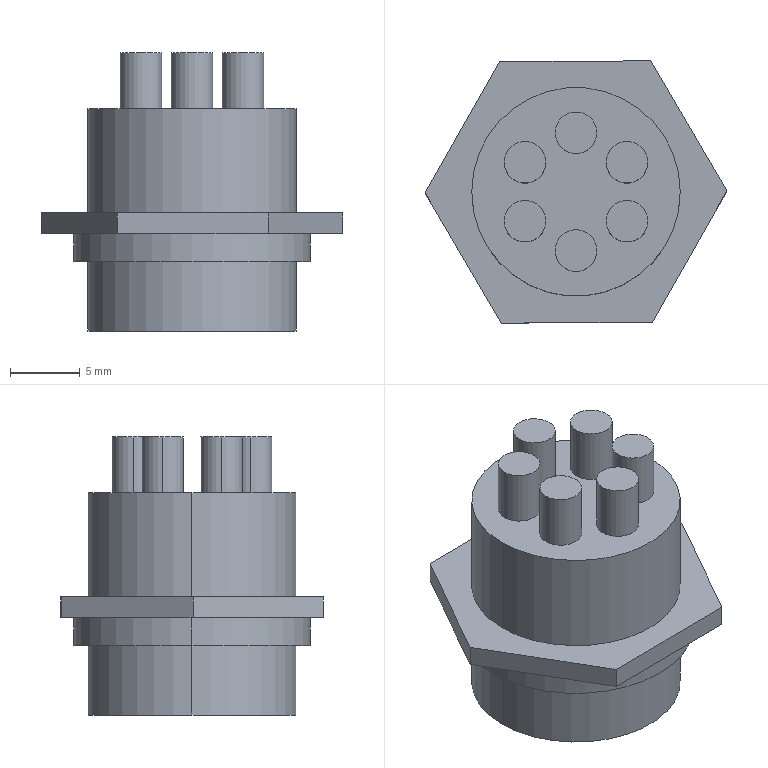Part | STEP file | 航插-1 | 1 solid | 56 faces | box 21.708 x 18.872 x 20 mm | volume 2692 mm3 | cylinder 32 | plane 24 | commonest cylinder face diameters 3 x24 15 x4 14 x2 17 x2
STEP:
#1=CARTESIAN_POINT('',(-7.5,0.,16.));
#2=VERTEX_POINT('',#1);
#3=CARTESIAN_POINT('',(7.5,0.,16.));
#4=VERTEX_POINT('',#3);
#5=CARTESIAN_POINT('',(0.,0.,16.));
#6=DIRECTION('',(0.,0.,-1.));
#7=DIRECTION('',(-1.,0.,0.));
#8=AXIS2_PLACEMENT_3D('',#5,#6,#7);
#9=CIRCLE('',#8,7.5);
#10=EDGE_CURVE('',#2,#4,#9,.T.);
#11=ORIENTED_EDGE('',*,*,#10,.T.);
#12=CARTESIAN_POINT('',(7.5,0.,8.5));
#13=VERTEX_POINT('',#12);
#14=CARTESIAN_POINT('',(7.5,0.,16.));
#15=DIRECTION('',(0.,0.,-1.));
#16=VECTOR('',#15,1000.);
#17=LINE('',#14,#16);
#18=EDGE_CURVE('',#4,#13,#17,.T.);
#19=ORIENTED_EDGE('',*,*,#18,.T.);
#20=CARTESIAN_POINT('',(-7.5,0.,8.5));
#21=VERTEX_POINT('',#20);
#22=CARTESIAN_POINT('',(0.,0.,8.5));
#23=DIRECTION('',(0.,0.,1.));
#24=DIRECTION('',(-1.,0.,0.));
#25=AXIS2_PLACEMENT_3D('',#22,#23,#24);
#26=CIRCLE('',#25,7.5);
#27=EDGE_CURVE('',#13,#21,#26,.T.);
#28=ORIENTED_EDGE('',*,*,#27,.T.);
#29=CARTESIAN_POINT('',(-7.5,0.,16.));
#30=DIRECTION('',(0.,0.,-1.));
#31=VECTOR('',#30,1000.);
#32=LINE('',#29,#31);
#33=EDGE_CURVE('',#2,#21,#32,.T.);
#34=ORIENTED_EDGE('',*,*,#33,.F.);
#35=EDGE_LOOP('',(#11,#19,#28,#34));
#36=FACE_OUTER_BOUND('',#35,.T.);
#37=CARTESIAN_POINT('',(0.,0.,16.));
#38=DIRECTION('',(0.,0.,-1.));
#39=DIRECTION('',(-1.,0.,0.));
#40=AXIS2_PLACEMENT_3D('',#37,#38,#39);
#41=CYLINDRICAL_SURFACE('',#40,7.5);
#42=ADVANCED_FACE('',(#36),#41,.T.);
#43=CARTESIAN_POINT('',(-5.17,2.119,20.));
#44=VERTEX_POINT('',#43);
#45=CARTESIAN_POINT('',(-2.17,2.119,20.));
#46=VERTEX_POINT('',#45);
#47=CARTESIAN_POINT('',(-3.67,2.119,20.));
#48=DIRECTION('',(0.,0.,-1.));
#49=DIRECTION('',(-1.,0.,0.));
#50=AXIS2_PLACEMENT_3D('',#47,#48,#49);
#51=CIRCLE('',#50,1.5);
#52=EDGE_CURVE('',#44,#46,#51,.T.);
#53=ORIENTED_EDGE('',*,*,#52,.T.);
#54=CARTESIAN_POINT('',(-2.17,2.119,16.));
#55=VERTEX_POINT('',#54);
#56=CARTESIAN_POINT('',(-2.17,2.119,20.));
#57=DIRECTION('',(0.,0.,-1.));
#58=VECTOR('',#57,1000.);
#59=LINE('',#56,#58);
#60=EDGE_CURVE('',#46,#55,#59,.T.);
#61=ORIENTED_EDGE('',*,*,#60,.T.);
#62=CARTESIAN_POINT('',(-5.17,2.119,16.));
#63=VERTEX_POINT('',#62);
#64=CARTESIAN_POINT('',(-3.67,2.119,16.));
#65=DIRECTION('',(0.,0.,-1.));
#66=DIRECTION('',(-1.,0.,0.));
#67=AXIS2_PLACEMENT_3D('',#64,#65,#66);
#68=CIRCLE('',#67,1.5);
#69=EDGE_CURVE('',#63,#55,#68,.T.);
#70=ORIENTED_EDGE('',*,*,#69,.F.);
#71=CARTESIAN_POINT('',(-5.17,2.119,20.));
#72=DIRECTION('',(0.,0.,-1.));
#73=VECTOR('',#72,1000.);
#74=LINE('',#71,#73);
#75=EDGE_CURVE('',#44,#63,#74,.T.);
#76=ORIENTED_EDGE('',*,*,#75,.F.);
#77=EDGE_LOOP('',(#53,#61,#70,#76));
#78=FACE_OUTER_BOUND('',#77,.T.);
#79=CARTESIAN_POINT('',(-3.67,2.119,20.));
#80=DIRECTION('',(0.,0.,-1.));
#81=DIRECTION('',(-1.,0.,0.));
#82=AXIS2_PLACEMENT_3D('',#79,#80,#81);
#83=CYLINDRICAL_SURFACE('',#82,1.5);
#84=ADVANCED_FACE('',(#78),#83,.T.);
#85=CARTESIAN_POINT('',(-5.17,-2.119,20.));
#86=VERTEX_POINT('',#85);
#87=CARTESIAN_POINT('',(-2.17,-2.119,20.));
#88=VERTEX_POINT('',#87);
#89=CARTESIAN_POINT('',(-3.67,-2.119,20.));
#90=DIRECTION('',(0.,0.,-1.));
#91=DIRECTION('',(-1.,0.,0.));
#92=AXIS2_PLACEMENT_3D('',#89,#90,#91);
#93=CIRCLE('',#92,1.5);
#94=EDGE_CURVE('',#86,#88,#93,.T.);
#95=ORIENTED_EDGE('',*,*,#94,.T.);
#96=CARTESIAN_POINT('',(-2.17,-2.119,16.));
#97=VERTEX_POINT('',#96);
#98=CARTESIAN_POINT('',(-2.17,-2.119,20.));
#99=DIRECTION('',(0.,0.,-1.));
#100=VECTOR('',#99,1000.);
#101=LINE('',#98,#100);
#102=EDGE_CURVE('',#88,#97,#101,.T.);
#103=ORIENTED_EDGE('',*,*,#102,.T.);
#104=CARTESIAN_POINT('',(-5.17,-2.119,16.));
#105=VERTEX_POINT('',#104);
#106=CARTESIAN_POINT('',(-3.67,-2.119,16.));
#107=DIRECTION('',(0.,0.,-1.));
#108=DIRECTION('',(-1.,0.,0.));
#109=AXIS2_PLACEMENT_3D('',#106,#107,#108);
#110=CIRCLE('',#109,1.5);
#111=EDGE_CURVE('',#105,#97,#110,.T.);
#112=ORIENTED_EDGE('',*,*,#111,.F.);
#113=CARTESIAN_POINT('',(-5.17,-2.119,20.));
#114=DIRECTION('',(0.,0.,-1.));
#115=VECTOR('',#114,1000.);
#116=LINE('',#113,#115);
#117=EDGE_CURVE('',#86,#105,#116,.T.);
#118=ORIENTED_EDGE('',*,*,#117,.F.);
#119=EDGE_LOOP('',(#95,#103,#112,#118));
#120=FACE_OUTER_BOUND('',#119,.T.);
#121=CARTESIAN_POINT('',(-3.67,-2.119,20.));
#122=DIRECTION('',(0.,0.,-1.));
#123=DIRECTION('',(-1.,0.,0.));
#124=AXIS2_PLACEMENT_3D('',#121,#122,#123);
#125=CYLINDRICAL_SURFACE('',#124,1.5);
#126=ADVANCED_FACE('',(#120),#125,.T.);
#127=CARTESIAN_POINT('',(-1.5,-4.238,20.));
#128=VERTEX_POINT('',#127);
#129=CARTESIAN_POINT('',(1.5,-4.238,20.));
#130=VERTEX_POINT('',#129);
#131=CARTESIAN_POINT('',(0.,-4.238,20.));
#132=DIRECTION('',(0.,0.,-1.));
#133=DIRECTION('',(-1.,0.,0.));
#134=AXIS2_PLACEMENT_3D('',#131,#132,#133);
#135=CIRCLE('',#134,1.5);
#136=EDGE_CURVE('',#128,#130,#135,.T.);
#137=ORIENTED_EDGE('',*,*,#136,.T.);
#138=CARTESIAN_POINT('',(1.5,-4.238,16.));
#139=VERTEX_POINT('',#138);
#140=CARTESIAN_POINT('',(1.5,-4.238,20.));
#141=DIRECTION('',(0.,0.,-1.));
#142=VECTOR('',#141,1000.);
#143=LINE('',#140,#142);
#144=EDGE_CURVE('',#130,#139,#143,.T.);
#145=ORIENTED_EDGE('',*,*,#144,.T.);
#146=CARTESIAN_POINT('',(-1.5,-4.238,16.));
#147=VERTEX_POINT('',#146);
#148=CARTESIAN_POINT('',(0.,-4.238,16.));
#149=DIRECTION('',(0.,0.,-1.));
#150=DIRECTION('',(-1.,0.,0.));
#151=AXIS2_PLACEMENT_3D('',#148,#149,#150);
#152=CIRCLE('',#151,1.5);
#153=EDGE_CURVE('',#147,#139,#152,.T.);
#154=ORIENTED_EDGE('',*,*,#153,.F.);
#155=CARTESIAN_POINT('',(-1.5,-4.238,20.));
#156=DIRECTION('',(0.,0.,-1.));
#157=VECTOR('',#156,1000.);
#158=LINE('',#155,#157);
#159=EDGE_CURVE('',#128,#147,#158,.T.);
#160=ORIENTED_EDGE('',*,*,#159,.F.);
#161=EDGE_LOOP('',(#137,#145,#154,#160));
#162=FACE_OUTER_BOUND('',#161,.T.);
#163=CARTESIAN_POINT('',(0.,-4.238,20.));
#164=DIRECTION('',(0.,0.,-1.));
#165=DIRECTION('',(-1.,0.,0.));
#166=AXIS2_PLACEMENT_3D('',#163,#164,#165);
#167=CYLINDRICAL_SURFACE('',#166,1.5);
#168=ADVANCED_FACE('',(#162),#167,.T.);
#169=CARTESIAN_POINT('',(2.17,-2.119,20.));
#170=VERTEX_POINT('',#169);
#171=CARTESIAN_POINT('',(5.17,-2.119,20.));
#172=VERTEX_POINT('',#171);
#173=CARTESIAN_POINT('',(3.67,-2.119,20.));
#174=DIRECTION('',(0.,0.,-1.));
#175=DIRECTION('',(-1.,0.,0.));
#176=AXIS2_PLACEMENT_3D('',#173,#174,#175);
#177=CIRCLE('',#176,1.5);
#178=EDGE_CURVE('',#170,#172,#177,.T.);
#179=ORIENTED_EDGE('',*,*,#178,.T.);
#180=CARTESIAN_POINT('',(5.17,-2.119,16.));
#181=VERTEX_POINT('',#180);
#182=CARTESIAN_POINT('',(5.17,-2.119,20.));
#183=DIRECTION('',(0.,0.,-1.));
#184=VECTOR('',#183,1000.);
#185=LINE('',#182,#184);
#186=EDGE_CURVE('',#172,#181,#185,.T.);
#187=ORIENTED_EDGE('',*,*,#186,.T.);
#188=CARTESIAN_POINT('',(2.17,-2.119,16.));
#189=VERTEX_POINT('',#188);
#190=CARTESIAN_POINT('',(3.67,-2.119,16.));
#191=DIRECTION('',(0.,0.,-1.));
#192=DIRECTION('',(-1.,0.,0.));
#193=AXIS2_PLACEMENT_3D('',#190,#191,#192);
#194=CIRCLE('',#193,1.5);
#195=EDGE_CURVE('',#189,#181,#194,.T.);
#196=ORIENTED_EDGE('',*,*,#195,.F.);
#197=CARTESIAN_POINT('',(2.17,-2.119,20.));
#198=DIRECTION('',(0.,0.,-1.));
#199=VECTOR('',#198,1000.);
#200=LINE('',#197,#199);
#201=EDGE_CURVE('',#170,#189,#200,.T.);
#202=ORIENTED_EDGE('',*,*,#201,.F.);
#203=EDGE_LOOP('',(#179,#187,#196,#202));
#204=FACE_OUTER_BOUND('',#203,.T.);
#205=CARTESIAN_POINT('',(3.67,-2.119,20.));
#206=DIRECTION('',(0.,0.,-1.));
#207=DIRECTION('',(-1.,0.,0.));
#208=AXIS2_PLACEMENT_3D('',#205,#206,#207);
#209=CYLINDRICAL_SURFACE('',#208,1.5);
#210=ADVANCED_FACE('',(#204),#209,.T.);
#211=CARTESIAN_POINT('',(2.17,2.119,20.));
#212=VERTEX_POINT('',#211);
#213=CARTESIAN_POINT('',(5.17,2.119,20.));
#214=VERTEX_POINT('',#213);
#215=CARTESIAN_POINT('',(3.67,2.119,20.));
#216=DIRECTION('',(0.,0.,-1.));
#217=DIRECTION('',(-1.,0.,0.));
#218=AXIS2_PLACEMENT_3D('',#215,#216,#217);
#219=CIRCLE('',#218,1.5);
#220=EDGE_CURVE('',#212,#214,#219,.T.);
#221=ORIENTED_EDGE('',*,*,#220,.T.);
#222=CARTESIAN_POINT('',(5.17,2.119,16.));
#223=VERTEX_POINT('',#222);
#224=CARTESIAN_POINT('',(5.17,2.119,20.));
#225=DIRECTION('',(0.,0.,-1.));
#226=VECTOR('',#225,1000.);
#227=LINE('',#224,#226);
#228=EDGE_CURVE('',#214,#223,#227,.T.);
#229=ORIENTED_EDGE('',*,*,#228,.T.);
#230=CARTESIAN_POINT('',(2.17,2.119,16.));
#231=VERTEX_POINT('',#230);
#232=CARTESIAN_POINT('',(3.67,2.119,16.));
#233=DIRECTION('',(0.,0.,-1.));
#234=DIRECTION('',(-1.,0.,0.));
#235=AXIS2_PLACEMENT_3D('',#232,#233,#234);
#236=CIRCLE('',#235,1.5);
#237=EDGE_CURVE('',#231,#223,#236,.T.);
#238=ORIENTED_EDGE('',*,*,#237,.F.);
#239=CARTESIAN_POINT('',(2.17,2.119,20.));
#240=DIRECTION('',(0.,0.,-1.));
#241=VECTOR('',#240,1000.);
#242=LINE('',#239,#241);
#243=EDGE_CURVE('',#212,#231,#242,.T.);
#244=ORIENTED_EDGE('',*,*,#243,.F.);
#245=EDGE_LOOP('',(#221,#229,#238,#244));
#246=FACE_OUTER_BOUND('',#245,.T.);
#247=CARTESIAN_POINT('',(3.67,2.119,20.));
#248=DIRECTION('',(0.,0.,-1.));
#249=DIRECTION('',(-1.,0.,0.));
#250=AXIS2_PLACEMENT_3D('',#247,#248,#249);
#251=CYLINDRICAL_SURFACE('',#250,1.5);
#252=ADVANCED_FACE('',(#246),#251,.T.);
#253=CARTESIAN_POINT('',(-1.5,4.238,20.));
#254=VERTEX_POINT('',#253);
#255=CARTESIAN_POINT('',(1.5,4.238,20.));
#256=VERTEX_POINT('',#255);
#257=CARTESIAN_POINT('',(0.,4.238,20.));
#258=DIRECTION('',(0.,0.,-1.));
#259=DIRECTION('',(-1.,0.,0.));
#260=AXIS2_PLACEMENT_3D('',#257,#258,#259);
#261=CIRCLE('',#260,1.5);
#262=EDGE_CURVE('',#254,#256,#261,.T.);
#263=ORIENTED_EDGE('',*,*,#262,.T.);
#264=CARTESIAN_POINT('',(1.5,4.238,16.));
#265=VERTEX_POINT('',#264);
#266=CARTESIAN_POINT('',(1.5,4.238,20.));
#267=DIRECTION('',(0.,0.,-1.));
#268=VECTOR('',#267,1000.);
#269=LINE('',#266,#268);
#270=EDGE_CURVE('',#256,#265,#269,.T.);
#271=ORIENTED_EDGE('',*,*,#270,.T.);
#272=CARTESIAN_POINT('',(-1.5,4.238,16.));
#273=VERTEX_POINT('',#272);
#274=CARTESIAN_POINT('',(0.,4.238,16.));
#275=DIRECTION('',(0.,0.,-1.));
#276=DIRECTION('',(-1.,0.,0.));
#277=AXIS2_PLACEMENT_3D('',#274,#275,#276);
#278=CIRCLE('',#277,1.5);
#279=EDGE_CURVE('',#273,#265,#278,.T.);
#280=ORIENTED_EDGE('',*,*,#279,.F.);
#281=CARTESIAN_POINT('',(-1.5,4.238,20.));
#282=DIRECTION('',(0.,0.,-1.));
#283=VECTOR('',#282,1000.);
#284=LINE('',#281,#283);
#285=EDGE_CURVE('',#254,#273,#284,.T.);
#286=ORIENTED_EDGE('',*,*,#285,.F.);
#287=EDGE_LOOP('',(#263,#271,#280,#286));
#288=FACE_OUTER_BOUND('',#287,.T.);
#289=CARTESIAN_POINT('',(0.,4.238,20.));
#290=DIRECTION('',(0.,0.,-1.));
#291=DIRECTION('',(-1.,0.,0.));
#292=AXIS2_PLACEMENT_3D('',#289,#290,#291);
#293=CYLINDRICAL_SURFACE('',#292,1.5);
#294=ADVANCED_FACE('',(#288),#293,.T.);
#295=CARTESIAN_POINT('',(-8.5,0.,7.));
#296=VERTEX_POINT('',#295);
#297=CARTESIAN_POINT('',(8.5,0.,7.));
#298=VERTEX_POINT('',#297);
#299=CARTESIAN_POINT('',(0.,0.,7.));
#300=DIRECTION('',(0.,0.,-1.));
#301=DIRECTION('',(-1.,0.,0.));
#302=AXIS2_PLACEMENT_3D('',#299,#300,#301);
#303=CIRCLE('',#302,8.5);
#304=EDGE_CURVE('',#296,#298,#303,.T.);
#305=ORIENTED_EDGE('',*,*,#304,.T.);
#306=CARTESIAN_POINT('',(8.5,0.,5.));
#307=VERTEX_POINT('',#306);
#308=CARTESIAN_POINT('',(8.5,0.,7.));
#309=DIRECTION('',(0.,0.,-1.));
#310=VECTOR('',#309,1000.);
#311=LINE('',#308,#310);
#312=EDGE_CURVE('',#298,#307,#311,.T.);
#313=ORIENTED_EDGE('',*,*,#312,.T.);
#314=CARTESIAN_POINT('',(-8.5,0.,5.));
#315=VERTEX_POINT('',#314);
#316=CARTESIAN_POINT('',(0.,0.,5.));
#317=DIRECTION('',(0.,0.,1.));
#318=DIRECTION('',(-1.,0.,0.));
#319=AXIS2_PLACEMENT_3D('',#316,#317,#318);
#320=CIRCLE('',#319,8.5);
#321=EDGE_CURVE('',#307,#315,#320,.T.);
#322=ORIENTED_EDGE('',*,*,#321,.T.);
#323=CARTESIAN_POINT('',(-8.5,0.,7.));
#324=DIRECTION('',(0.,0.,-1.));
#325=VECTOR('',#324,1000.);
#326=LINE('',#323,#325);
#327=EDGE_CURVE('',#296,#315,#326,.T.);
#328=ORIENTED_EDGE('',*,*,#327,.F.);
#329=EDGE_LOOP('',(#305,#313,#322,#328));
#330=FACE_OUTER_BOUND('',#329,.T.);
#331=CARTESIAN_POINT('',(0.,0.,7.));
#332=DIRECTION('',(0.,0.,-1.));
#333=DIRECTION('',(-1.,0.,0.));
#334=AXIS2_PLACEMENT_3D('',#331,#332,#333);
#335=CYLINDRICAL_SURFACE('',#334,8.5);
#336=ADVANCED_FACE('',(#330),#335,.T.);
#337=CARTESIAN_POINT('',(-7.5,0.,5.));
#338=VERTEX_POINT('',#337);
#339=CARTESIAN_POINT('',(7.5,0.,5.));
#340=VERTEX_POINT('',#339);
#341=CARTESIAN_POINT('',(0.,0.,5.));
#342=DIRECTION('',(0.,0.,-1.));
#343=DIRECTION('',(-1.,0.,0.));
#344=AXIS2_PLACEMENT_3D('',#341,#342,#343);
#345=CIRCLE('',#344,7.5);
#346=EDGE_CURVE('',#338,#340,#345,.T.);
#347=ORIENTED_EDGE('',*,*,#346,.T.);
#348=CARTESIAN_POINT('',(7.5,0.,0.));
#349=VERTEX_POINT('',#348);
#350=CARTESIAN_POINT('',(7.5,0.,5.));
#351=DIRECTION('',(0.,0.,-1.));
#352=VECTOR('',#351,1000.);
#353=LINE('',#350,#352);
#354=EDGE_CURVE('',#340,#349,#353,.T.);
#355=ORIENTED_EDGE('',*,*,#354,.T.);
#356=CARTESIAN_POINT('',(-7.5,0.,0.));
#357=VERTEX_POINT('',#356);
#358=CARTESIAN_POINT('',(0.,0.,0.));
#359=DIRECTION('',(0.,0.,1.));
#360=DIRECTION('',(-1.,0.,0.));
#361=AXIS2_PLACEMENT_3D('',#358,#359,#360);
#362=CIRCLE('',#361,7.5);
#363=EDGE_CURVE('',#349,#357,#362,.T.);
#364=ORIENTED_EDGE('',*,*,#363,.T.);
#365=CARTESIAN_POINT('',(-7.5,0.,5.));
#366=DIRECTION('',(0.,0.,-1.));
#367=VECTOR('',#366,1000.);
#368=LINE('',#365,#367);
#369=EDGE_CURVE('',#338,#357,#368,.T.);
#370=ORIENTED_EDGE('',*,*,#369,.F.);
#371=EDGE_LOOP('',(#347,#355,#364,#370));
#372=FACE_OUTER_BOUND('',#371,.T.);
#373=CARTESIAN_POINT('',(0.,0.,5.));
#374=DIRECTION('',(0.,0.,-1.));
#375=DIRECTION('',(-1.,0.,0.));
#376=AXIS2_PLACEMENT_3D('',#373,#374,#375);
#377=CYLINDRICAL_SURFACE('',#376,7.5);
#378=ADVANCED_FACE('',(#372),#377,.T.);
#379=CARTESIAN_POINT('',(7.,0.,5.));
#380=VERTEX_POINT('',#379);
#381=CARTESIAN_POINT('',(-7.,0.,5.));
#382=VERTEX_POINT('',#381);
#383=CARTESIAN_POINT('',(0.,0.,5.));
#384=DIRECTION('',(0.,0.,-1.));
#385=DIRECTION('',(-1.,0.,0.));
#386=AXIS2_PLACEMENT_3D('',#383,#384,#385);
#387=CIRCLE('',#386,7.);
#388=EDGE_CURVE('',#380,#382,#387,.T.);
#389=ORIENTED_EDGE('',*,*,#388,.F.);
#390=CARTESIAN_POINT('',(7.,0.,0.));
#391=VERTEX_POINT('',#390);
#392=CARTESIAN_POINT('',(7.,0.,5.));
#393=DIRECTION('',(0.,0.,-1.));
#394=VECTOR('',#393,1000.);
#395=LINE('',#392,#394);
#396=EDGE_CURVE('',#380,#391,#395,.T.);
#397=ORIENTED_EDGE('',*,*,#396,.T.);
#398=CARTESIAN_POINT('',(-7.,0.,0.));
#399=VERTEX_POINT('',#398);
#400=CARTESIAN_POINT('',(0.,0.,0.));
#401=DIRECTION('',(0.,0.,-1.));
#402=DIRECTION('',(-1.,0.,0.));
#403=AXIS2_PLACEMENT_3D('',#400,#401,#402);
#404=CIRCLE('',#403,7.);
#405=EDGE_CURVE('',#391,#399,#404,.T.);
#406=ORIENTED_EDGE('',*,*,#405,.T.);
#407=CARTESIAN_POINT('',(-7.,0.,5.));
#408=DIRECTION('',(0.,0.,-1.));
#409=VECTOR('',#408,1000.);
#410=LINE('',#407,#409);
#411=EDGE_CURVE('',#382,#399,#410,.T.);
#412=ORIENTED_EDGE('',*,*,#411,.F.);
#413=EDGE_LOOP('',(#389,#397,#406,#412));
#414=FACE_OUTER_BOUND('',#413,.T.);
#415=CARTESIAN_POINT('',(0.,0.,5.));
#416=DIRECTION('',(0.,0.,-1.));
#417=DIRECTION('',(-1.,0.,0.));
#418=AXIS2_PLACEMENT_3D('',#415,#416,#417);
#419=CYLINDRICAL_SURFACE('',#418,7.);
#420=ADVANCED_FACE('',(#414),#419,.F.);
#421=CARTESIAN_POINT('',(-1.637,1.811,1.));
#422=VERTEX_POINT('',#421);
#423=CARTESIAN_POINT('',(-4.637,1.811,1.));
#424=VERTEX_POINT('',#423);
#425=CARTESIAN_POINT('',(-3.137,1.811,1.));
#426=DIRECTION('',(0.,0.,1.));
#427=DIRECTION('',(1.,0.,0.));
#428=AXIS2_PLACEMENT_3D('',#425,#426,#427);
#429=CIRCLE('',#428,1.5);
#430=EDGE_CURVE('',#422,#424,#429,.T.);
#431=ORIENTED_EDGE('',*,*,#430,.T.);
#432=CARTESIAN_POINT('',(-4.637,1.811,5.));
#433=VERTEX_POINT('',#432);
#434=CARTESIAN_POINT('',(-4.637,1.811,1.));
#435=DIRECTION('',(0.,0.,1.));
#436=VECTOR('',#435,1000.);
#437=LINE('',#434,#436);
#438=EDGE_CURVE('',#424,#433,#437,.T.);
#439=ORIENTED_EDGE('',*,*,#438,.T.);
#440=CARTESIAN_POINT('',(-1.637,1.811,5.));
#441=VERTEX_POINT('',#440);
#442=CARTESIAN_POINT('',(-3.137,1.811,5.));
#443=DIRECTION('',(0.,0.,-1.));
#444=DIRECTION('',(1.,0.,0.));
#445=AXIS2_PLACEMENT_3D('',#442,#443,#444);
#446=CIRCLE('',#445,1.5);
#447=EDGE_CURVE('',#433,#441,#446,.T.);
#448=ORIENTED_EDGE('',*,*,#447,.T.);
#449=CARTESIAN_POINT('',(-1.637,1.811,1.));
#450=DIRECTION('',(0.,0.,1.));
#451=VECTOR('',#450,1000.);
#452=LINE('',#449,#451);
#453=EDGE_CURVE('',#422,#441,#452,.T.);
#454=ORIENTED_EDGE('',*,*,#453,.F.);
#455=EDGE_LOOP('',(#431,#439,#448,#454));
#456=FACE_OUTER_BOUND('',#455,.T.);
#457=CARTESIAN_POINT('',(-3.137,1.811,1.));
#458=DIRECTION('',(0.,0.,1.));
#459=DIRECTION('',(1.,0.,0.));
#460=AXIS2_PLACEMENT_3D('',#457,#458,#459);
#461=CYLINDRICAL_SURFACE('',#460,1.5);
#462=ADVANCED_FACE('',(#456),#461,.T.);
#463=CARTESIAN_POINT('',(-1.637,-1.811,1.));
#464=VERTEX_POINT('',#463);
#465=CARTESIAN_POINT('',(-4.637,-1.811,1.));
#466=VERTEX_POINT('',#465);
#467=CARTESIAN_POINT('',(-3.137,-1.811,1.));
#468=DIRECTION('',(0.,0.,1.));
#469=DIRECTION('',(1.,0.,0.));
#470=AXIS2_PLACEMENT_3D('',#467,#468,#469);
#471=CIRCLE('',#470,1.5);
#472=EDGE_CURVE('',#464,#466,#471,.T.);
#473=ORIENTED_EDGE('',*,*,#472,.T.);
#474=CARTESIAN_POINT('',(-4.637,-1.811,5.));
#475=VERTEX_POINT('',#474);
#476=CARTESIAN_POINT('',(-4.637,-1.811,1.));
#477=DIRECTION('',(0.,0.,1.));
#478=VECTOR('',#477,1000.);
#479=LINE('',#476,#478);
#480=EDGE_CURVE('',#466,#475,#479,.T.);
#481=ORIENTED_EDGE('',*,*,#480,.T.);
#482=CARTESIAN_POINT('',(-1.637,-1.811,5.));
#483=VERTEX_POINT('',#482);
#484=CARTESIAN_POINT('',(-3.137,-1.811,5.));
#485=DIRECTION('',(0.,0.,-1.));
#486=DIRECTION('',(1.,0.,0.));
#487=AXIS2_PLACEMENT_3D('',#484,#485,#486);
#488=CIRCLE('',#487,1.5);
#489=EDGE_CURVE('',#475,#483,#488,.T.);
#490=ORIENTED_EDGE('',*,*,#489,.T.);
#491=CARTESIAN_POINT('',(-1.637,-1.811,1.));
#492=DIRECTION('',(0.,0.,1.));
#493=VECTOR('',#492,1000.);
#494=LINE('',#491,#493);
#495=EDGE_CURVE('',#464,#483,#494,.T.);
#496=ORIENTED_EDGE('',*,*,#495,.F.);
#497=EDGE_LOOP('',(#473,#481,#490,#496));
#498=FACE_OUTER_BOUND('',#497,.T.);
#499=CARTESIAN_POINT('',(-3.137,-1.811,1.));
#500=DIRECTION('',(0.,0.,1.));
#501=DIRECTION('',(1.,0.,0.));
#502=AXIS2_PLACEMENT_3D('',#499,#500,#501);
#503=CYLINDRICAL_SURFACE('',#502,1.5);
#504=ADVANCED_FACE('',(#498),#503,.T.);
#505=CARTESIAN_POINT('',(1.5,-3.623,1.));
#506=VERTEX_POINT('',#505);
#507=CARTESIAN_POINT('',(-1.5,-3.623,1.));
#508=VERTEX_POINT('',#507);
#509=CARTESIAN_POINT('',(0.,-3.623,1.));
#510=DIRECTION('',(0.,0.,1.));
#511=DIRECTION('',(1.,0.,0.));
#512=AXIS2_PLACEMENT_3D('',#509,#510,#511);
#513=CIRCLE('',#512,1.5);
#514=EDGE_CURVE('',#506,#508,#513,.T.);
#515=ORIENTED_EDGE('',*,*,#514,.T.);
#516=CARTESIAN_POINT('',(-1.5,-3.623,5.));
#517=VERTEX_POINT('',#516);
#518=CARTESIAN_POINT('',(-1.5,-3.623,1.));
#519=DIRECTION('',(0.,0.,1.));
#520=VECTOR('',#519,1000.);
#521=LINE('',#518,#520);
#522=EDGE_CURVE('',#508,#517,#521,.T.);
#523=ORIENTED_EDGE('',*,*,#522,.T.);
#524=CARTESIAN_POINT('',(1.5,-3.623,5.));
#525=VERTEX_POINT('',#524);
#526=CARTESIAN_POINT('',(0.,-3.623,5.));
#527=DIRECTION('',(0.,0.,-1.));
#528=DIRECTION('',(1.,0.,0.));
#529=AXIS2_PLACEMENT_3D('',#526,#527,#528);
#530=CIRCLE('',#529,1.5);
#531=EDGE_CURVE('',#517,#525,#530,.T.);
#532=ORIENTED_EDGE('',*,*,#531,.T.);
#533=CARTESIAN_POINT('',(1.5,-3.623,1.));
#534=DIRECTION('',(0.,0.,1.));
#535=VECTOR('',#534,1000.);
#536=LINE('',#533,#535);
#537=EDGE_CURVE('',#506,#525,#536,.T.);
#538=ORIENTED_EDGE('',*,*,#537,.F.);
#539=EDGE_LOOP('',(#515,#523,#532,#538));
#540=FACE_OUTER_BOUND('',#539,.T.);
#541=CARTESIAN_POINT('',(0.,-3.623,1.));
#542=DIRECTION('',(0.,0.,1.));
#543=DIRECTION('',(1.,0.,0.));
#544=AXIS2_PLACEMENT_3D('',#541,#542,#543);
#545=CYLINDRICAL_SURFACE('',#544,1.5);
#546=ADVANCED_FACE('',(#540),#545,.T.);
#547=CARTESIAN_POINT('',(4.637,-1.811,1.));
#548=VERTEX_POINT('',#547);
#549=CARTESIAN_POINT('',(1.637,-1.811,1.));
#550=VERTEX_POINT('',#549);
#551=CARTESIAN_POINT('',(3.137,-1.811,1.));
#552=DIRECTION('',(0.,0.,1.));
#553=DIRECTION('',(1.,0.,0.));
#554=AXIS2_PLACEMENT_3D('',#551,#552,#553);
#555=CIRCLE('',#554,1.5);
#556=EDGE_CURVE('',#548,#550,#555,.T.);
#557=ORIENTED_EDGE('',*,*,#556,.T.);
#558=CARTESIAN_POINT('',(1.637,-1.811,5.));
#559=VERTEX_POINT('',#558);
#560=CARTESIAN_POINT('',(1.637,-1.811,1.));
#561=DIRECTION('',(0.,0.,1.));
#562=VECTOR('',#561,1000.);
#563=LINE('',#560,#562);
#564=EDGE_CURVE('',#550,#559,#563,.T.);
#565=ORIENTED_EDGE('',*,*,#564,.T.);
#566=CARTESIAN_POINT('',(4.637,-1.811,5.));
#567=VERTEX_POINT('',#566);
#568=CARTESIAN_POINT('',(3.137,-1.811,5.));
#569=DIRECTION('',(0.,0.,-1.));
#570=DIRECTION('',(1.,0.,0.));
#571=AXIS2_PLACEMENT_3D('',#568,#569,#570);
#572=CIRCLE('',#571,1.5);
#573=EDGE_CURVE('',#559,#567,#572,.T.);
#574=ORIENTED_EDGE('',*,*,#573,.T.);
#575=CARTESIAN_POINT('',(4.637,-1.811,1.));
#576=DIRECTION('',(0.,0.,1.));
#577=VECTOR('',#576,1000.);
#578=LINE('',#575,#577);
#579=EDGE_CURVE('',#548,#567,#578,.T.);
#580=ORIENTED_EDGE('',*,*,#579,.F.);
#581=EDGE_LOOP('',(#557,#565,#574,#580));
#582=FACE_OUTER_BOUND('',#581,.T.);
#583=CARTESIAN_POINT('',(3.137,-1.811,1.));
#584=DIRECTION('',(0.,0.,1.));
#585=DIRECTION('',(1.,0.,0.));
#586=AXIS2_PLACEMENT_3D('',#583,#584,#585);
#587=CYLINDRICAL_SURFACE('',#586,1.5);
#588=ADVANCED_FACE('',(#582),#587,.T.);
#589=CARTESIAN_POINT('',(4.637,1.811,1.));
#590=VERTEX_POINT('',#589);
#591=CARTESIAN_POINT('',(1.637,1.811,1.));
#592=VERTEX_POINT('',#591);
#593=CARTESIAN_POINT('',(3.137,1.811,1.));
#594=DIRECTION('',(0.,0.,1.));
#595=DIRECTION('',(1.,0.,0.));
#596=AXIS2_PLACEMENT_3D('',#593,#594,#595);
#597=CIRCLE('',#596,1.5);
#598=EDGE_CURVE('',#590,#592,#597,.T.);
#599=ORIENTED_EDGE('',*,*,#598,.T.);
#600=CARTESIAN_POINT('',(1.637,1.811,5.));
#601=VERTEX_POINT('',#600);
#602=CARTESIAN_POINT('',(1.637,1.811,1.));
#603=DIRECTION('',(0.,0.,1.));
#604=VECTOR('',#603,1000.);
#605=LINE('',#602,#604);
#606=EDGE_CURVE('',#592,#601,#605,.T.);
#607=ORIENTED_EDGE('',*,*,#606,.T.);
#608=CARTESIAN_POINT('',(4.637,1.811,5.));
#609=VERTEX_POINT('',#608);
#610=CARTESIAN_POINT('',(3.137,1.811,5.));
#611=DIRECTION('',(0.,0.,-1.));
#612=DIRECTION('',(1.,0.,0.));
#613=AXIS2_PLACEMENT_3D('',#610,#611,#612);
#614=CIRCLE('',#613,1.5);
#615=EDGE_CURVE('',#601,#609,#614,.T.);
#616=ORIENTED_EDGE('',*,*,#615,.T.);
#617=CARTESIAN_POINT('',(4.637,1.811,1.));
#618=DIRECTION('',(0.,0.,1.));
#619=VECTOR('',#618,1000.);
#620=LINE('',#617,#619);
#621=EDGE_CURVE('',#590,#609,#620,.T.);
#622=ORIENTED_EDGE('',*,*,#621,.F.);
#623=EDGE_LOOP('',(#599,#607,#616,#622));
#624=FACE_OUTER_BOUND('',#623,.T.);
#625=CARTESIAN_POINT('',(3.137,1.811,1.));
#626=DIRECTION('',(0.,0.,1.));
#627=DIRECTION('',(1.,0.,0.));
#628=AXIS2_PLACEMENT_3D('',#625,#626,#627);
#629=CYLINDRICAL_SURFACE('',#628,1.5);
#630=ADVANCED_FACE('',(#624),#629,.T.);
#631=CARTESIAN_POINT('',(1.5,3.623,1.));
#632=VERTEX_POINT('',#631);
#633=CARTESIAN_POINT('',(-1.5,3.623,1.));
#634=VERTEX_POINT('',#633);
#635=CARTESIAN_POINT('',(0.,3.623,1.));
#636=DIRECTION('',(0.,0.,1.));
#637=DIRECTION('',(1.,0.,0.));
#638=AXIS2_PLACEMENT_3D('',#635,#636,#637);
#639=CIRCLE('',#638,1.5);
#640=EDGE_CURVE('',#632,#634,#639,.T.);
#641=ORIENTED_EDGE('',*,*,#640,.T.);
#642=CARTESIAN_POINT('',(-1.5,3.623,5.));
#643=VERTEX_POINT('',#642);
#644=CARTESIAN_POINT('',(-1.5,3.623,1.));
#645=DIRECTION('',(0.,0.,1.));
#646=VECTOR('',#645,1000.);
#647=LINE('',#644,#646);
#648=EDGE_CURVE('',#634,#643,#647,.T.);
#649=ORIENTED_EDGE('',*,*,#648,.T.);
#650=CARTESIAN_POINT('',(1.5,3.623,5.));
#651=VERTEX_POINT('',#650);
#652=CARTESIAN_POINT('',(0.,3.623,5.));
#653=DIRECTION('',(0.,0.,-1.));
#654=DIRECTION('',(1.,0.,0.));
#655=AXIS2_PLACEMENT_3D('',#652,#653,#654);
#656=CIRCLE('',#655,1.5);
#657=EDGE_CURVE('',#643,#651,#656,.T.);
#658=ORIENTED_EDGE('',*,*,#657,.T.);
#659=CARTESIAN_POINT('',(1.5,3.623,1.));
#660=DIRECTION('',(0.,0.,1.));
#661=VECTOR('',#660,1000.);
#662=LINE('',#659,#661);
#663=EDGE_CURVE('',#632,#651,#662,.T.);
#664=ORIENTED_EDGE('',*,*,#663,.F.);
#665=EDGE_LOOP('',(#641,#649,#658,#664));
#666=FACE_OUTER_BOUND('',#665,.T.);
#667=CARTESIAN_POINT('',(0.,3.623,1.));
#668=DIRECTION('',(0.,0.,1.));
#669=DIRECTION('',(1.,0.,0.));
#670=AXIS2_PLACEMENT_3D('',#667,#668,#669);
#671=CYLINDRICAL_SURFACE('',#670,1.5);
#672=ADVANCED_FACE('',(#666),#671,.T.);
#673=ORIENTED_EDGE('',*,*,#18,.F.);
#674=CARTESIAN_POINT('',(0.,0.,16.));
#675=DIRECTION('',(0.,0.,-1.));
#676=DIRECTION('',(-1.,0.,0.));
#677=AXIS2_PLACEMENT_3D('',#674,#675,#676);
#678=CIRCLE('',#677,7.5);
#679=EDGE_CURVE('',#4,#2,#678,.T.);
#680=ORIENTED_EDGE('',*,*,#679,.T.);
#681=ORIENTED_EDGE('',*,*,#33,.T.);
#682=CARTESIAN_POINT('',(0.,0.,8.5));
#683=DIRECTION('',(0.,0.,1.));
#684=DIRECTION('',(-1.,0.,0.));
#685=AXIS2_PLACEMENT_3D('',#682,#683,#684);
#686=CIRCLE('',#685,7.5);
#687=EDGE_CURVE('',#21,#13,#686,.T.);
#688=ORIENTED_EDGE('',*,*,#687,.T.);
#689=EDGE_LOOP('',(#673,#680,#681,#688));
#690=FACE_OUTER_BOUND('',#689,.T.);
#691=CARTESIAN_POINT('',(0.,0.,16.));
#692=DIRECTION('',(0.,0.,-1.));
#693=DIRECTION('',(-1.,0.,0.));
#694=AXIS2_PLACEMENT_3D('',#691,#692,#693);
#695=CYLINDRICAL_SURFACE('',#694,7.5);
#696=ADVANCED_FACE('',(#690),#695,.T.);
#697=ORIENTED_EDGE('',*,*,#687,.F.);
#698=ORIENTED_EDGE('',*,*,#27,.F.);
#699=EDGE_LOOP('',(#697,#698));
#700=FACE_BOUND('',#699,.T.);
#701=CARTESIAN_POINT('',(-5.49,9.364,8.5));
#702=VERTEX_POINT('',#701);
#703=CARTESIAN_POINT('',(-10.854,-0.07231,8.5));
#704=VERTEX_POINT('',#703);
#705=CARTESIAN_POINT('',(-5.49,9.364,8.5));
#706=DIRECTION('',(-0.4942,-0.8693,0.));
#707=VECTOR('',#706,1000.);
#708=LINE('',#705,#707);
#709=EDGE_CURVE('',#702,#704,#708,.T.);
#710=ORIENTED_EDGE('',*,*,#709,.T.);
#711=CARTESIAN_POINT('',(-5.364,-9.436,8.5));
#712=VERTEX_POINT('',#711);
#713=CARTESIAN_POINT('',(-10.854,-0.07231,8.5));
#714=DIRECTION('',(0.5058,-0.8627,0.));
#715=VECTOR('',#714,1000.);
#716=LINE('',#713,#715);
#717=EDGE_CURVE('',#704,#712,#716,.T.);
#718=ORIENTED_EDGE('',*,*,#717,.T.);
#719=CARTESIAN_POINT('',(5.49,-9.364,8.5));
#720=VERTEX_POINT('',#719);
#721=CARTESIAN_POINT('',(-5.364,-9.436,8.5));
#722=DIRECTION('',(1.,0.006662,0.));
#723=VECTOR('',#722,1000.);
#724=LINE('',#721,#723);
#725=EDGE_CURVE('',#712,#720,#724,.T.);
#726=ORIENTED_EDGE('',*,*,#725,.T.);
#727=CARTESIAN_POINT('',(10.854,0.07231,8.5));
#728=VERTEX_POINT('',#727);
#729=CARTESIAN_POINT('',(5.49,-9.364,8.5));
#730=DIRECTION('',(0.4942,0.8693,0.));
#731=VECTOR('',#730,1000.);
#732=LINE('',#729,#731);
#733=EDGE_CURVE('',#720,#728,#732,.T.);
#734=ORIENTED_EDGE('',*,*,#733,.T.);
#735=CARTESIAN_POINT('',(5.364,9.436,8.5));
#736=VERTEX_POINT('',#735);
#737=CARTESIAN_POINT('',(10.854,0.07231,8.5));
#738=DIRECTION('',(-0.5058,0.8627,0.));
#739=VECTOR('',#738,1000.);
#740=LINE('',#737,#739);
#741=EDGE_CURVE('',#728,#736,#740,.T.);
#742=ORIENTED_EDGE('',*,*,#741,.T.);
#743=CARTESIAN_POINT('',(5.364,9.436,8.5));
#744=DIRECTION('',(-1.,-0.006662,0.));
#745=VECTOR('',#744,1000.);
#746=LINE('',#743,#745);
#747=EDGE_CURVE('',#736,#702,#746,.T.);
#748=ORIENTED_EDGE('',*,*,#747,.T.);
#749=EDGE_LOOP('',(#710,#718,#726,#734,#742,#748));
#750=FACE_OUTER_BOUND('',#749,.T.);
#751=CARTESIAN_POINT('',(0.,0.,8.5));
#752=DIRECTION('',(0.,0.,1.));
#753=DIRECTION('',(1.,0.,0.));
#754=AXIS2_PLACEMENT_3D('',#751,#752,#753);
#755=PLANE('',#754);
#756=ADVANCED_FACE('',(#700,#750),#755,.T.);
#757=ORIENTED_EDGE('',*,*,#69,.T.);
#758=CARTESIAN_POINT('',(-3.67,2.119,16.));
#759=DIRECTION('',(0.,0.,-1.));
#760=DIRECTION('',(-1.,0.,0.));
#761=AXIS2_PLACEMENT_3D('',#758,#759,#760);
#762=CIRCLE('',#761,1.5);
#763=EDGE_CURVE('',#55,#63,#762,.T.);
#764=ORIENTED_EDGE('',*,*,#763,.T.);
#765=EDGE_LOOP('',(#757,#764));
#766=FACE_BOUND('',#765,.T.);
#767=ORIENTED_EDGE('',*,*,#111,.T.);
#768=CARTESIAN_POINT('',(-3.67,-2.119,16.));
#769=DIRECTION('',(0.,0.,-1.));
#770=DIRECTION('',(-1.,0.,0.));
#771=AXIS2_PLACEMENT_3D('',#768,#769,#770);
#772=CIRCLE('',#771,1.5);
#773=EDGE_CURVE('',#97,#105,#772,.T.);
#774=ORIENTED_EDGE('',*,*,#773,.T.);
#775=EDGE_LOOP('',(#767,#774));
#776=FACE_BOUND('',#775,.T.);
#777=ORIENTED_EDGE('',*,*,#153,.T.);
#778=CARTESIAN_POINT('',(0.,-4.238,16.));
#779=DIRECTION('',(0.,0.,-1.));
#780=DIRECTION('',(-1.,0.,0.));
#781=AXIS2_PLACEMENT_3D('',#778,#779,#780);
#782=CIRCLE('',#781,1.5);
#783=EDGE_CURVE('',#139,#147,#782,.T.);
#784=ORIENTED_EDGE('',*,*,#783,.T.);
#785=EDGE_LOOP('',(#777,#784));
#786=FACE_BOUND('',#785,.T.);
#787=ORIENTED_EDGE('',*,*,#195,.T.);
#788=CARTESIAN_POINT('',(3.67,-2.119,16.));
#789=DIRECTION('',(0.,0.,-1.));
#790=DIRECTION('',(-1.,0.,0.));
#791=AXIS2_PLACEMENT_3D('',#788,#789,#790);
#792=CIRCLE('',#791,1.5);
#793=EDGE_CURVE('',#181,#189,#792,.T.);
#794=ORIENTED_EDGE('',*,*,#793,.T.);
#795=EDGE_LOOP('',(#787,#794));
#796=FACE_BOUND('',#795,.T.);
#797=ORIENTED_EDGE('',*,*,#237,.T.);
#798=CARTESIAN_POINT('',(3.67,2.119,16.));
#799=DIRECTION('',(0.,0.,-1.));
#800=DIRECTION('',(-1.,0.,0.));
#801=AXIS2_PLACEMENT_3D('',#798,#799,#800);
#802=CIRCLE('',#801,1.5);
#803=EDGE_CURVE('',#223,#231,#802,.T.);
#804=ORIENTED_EDGE('',*,*,#803,.T.);
#805=EDGE_LOOP('',(#797,#804));
#806=FACE_BOUND('',#805,.T.);
#807=ORIENTED_EDGE('',*,*,#279,.T.);
#808=CARTESIAN_POINT('',(0.,4.238,16.));
#809=DIRECTION('',(0.,0.,-1.));
#810=DIRECTION('',(-1.,0.,0.));
#811=AXIS2_PLACEMENT_3D('',#808,#809,#810);
#812=CIRCLE('',#811,1.5);
#813=EDGE_CURVE('',#265,#273,#812,.T.);
#814=ORIENTED_EDGE('',*,*,#813,.T.);
#815=EDGE_LOOP('',(#807,#814));
#816=FACE_BOUND('',#815,.T.);
#817=ORIENTED_EDGE('',*,*,#10,.F.);
#818=ORIENTED_EDGE('',*,*,#679,.F.);
#819=EDGE_LOOP('',(#817,#818));
#820=FACE_OUTER_BOUND('',#819,.T.);
#821=CARTESIAN_POINT('',(0.,0.,16.));
#822=DIRECTION('',(0.,0.,1.));
#823=DIRECTION('',(1.,0.,0.));
#824=AXIS2_PLACEMENT_3D('',#821,#822,#823);
#825=PLANE('',#824);
#826=ADVANCED_FACE('',(#766,#776,#786,#796,#806,#816,#820),#825,.T.);
#827=ORIENTED_EDGE('',*,*,#717,.F.);
#828=CARTESIAN_POINT('',(-10.854,-0.07231,7.));
#829=VERTEX_POINT('',#828);
#830=CARTESIAN_POINT('',(-10.854,-0.07231,8.5));
#831=DIRECTION('',(0.,0.,1.));
#832=VECTOR('',#831,1000.);
#833=LINE('',#830,#832);
#834=EDGE_CURVE('',#829,#704,#833,.T.);
#835=ORIENTED_EDGE('',*,*,#834,.F.);
#836=CARTESIAN_POINT('',(-5.364,-9.436,7.));
#837=VERTEX_POINT('',#836);
#838=CARTESIAN_POINT('',(-10.854,-0.07231,7.));
#839=DIRECTION('',(-0.5058,0.8627,0.));
#840=VECTOR('',#839,1000.);
#841=LINE('',#838,#840);
#842=EDGE_CURVE('',#837,#829,#841,.T.);
#843=ORIENTED_EDGE('',*,*,#842,.F.);
#844=CARTESIAN_POINT('',(-5.364,-9.436,8.5));
#845=DIRECTION('',(0.,0.,-1.));
#846=VECTOR('',#845,1000.);
#847=LINE('',#844,#846);
#848=EDGE_CURVE('',#712,#837,#847,.T.);
#849=ORIENTED_EDGE('',*,*,#848,.F.);
#850=EDGE_LOOP('',(#827,#835,#843,#849));
#851=FACE_OUTER_BOUND('',#850,.T.);
#852=CARTESIAN_POINT('',(-10.854,-0.07231,8.5));
#853=DIRECTION('',(0.8627,0.5058,0.));
#854=DIRECTION('',(-0.5058,0.8627,0.));
#855=AXIS2_PLACEMENT_3D('',#852,#853,#854);
#856=PLANE('',#855);
#857=ADVANCED_FACE('',(#851),#856,.F.);
#858=ORIENTED_EDGE('',*,*,#709,.F.);
#859=CARTESIAN_POINT('',(-5.49,9.364,7.));
#860=VERTEX_POINT('',#859);
#861=CARTESIAN_POINT('',(-5.49,9.364,8.5));
#862=DIRECTION('',(0.,0.,1.));
#863=VECTOR('',#862,1000.);
#864=LINE('',#861,#863);
#865=EDGE_CURVE('',#860,#702,#864,.T.);
#866=ORIENTED_EDGE('',*,*,#865,.F.);
#867=CARTESIAN_POINT('',(-5.49,9.364,7.));
#868=DIRECTION('',(0.4942,0.8693,0.));
#869=VECTOR('',#868,1000.);
#870=LINE('',#867,#869);
#871=EDGE_CURVE('',#829,#860,#870,.T.);
#872=ORIENTED_EDGE('',*,*,#871,.F.);
#873=ORIENTED_EDGE('',*,*,#834,.T.);
#874=EDGE_LOOP('',(#858,#866,#872,#873));
#875=FACE_OUTER_BOUND('',#874,.T.);
#876=CARTESIAN_POINT('',(-5.49,9.364,8.5));
#877=DIRECTION('',(0.8693,-0.4942,0.));
#878=DIRECTION('',(0.4942,0.8693,0.));
#879=AXIS2_PLACEMENT_3D('',#876,#877,#878);
#880=PLANE('',#879);
#881=ADVANCED_FACE('',(#875),#880,.F.);
#882=ORIENTED_EDGE('',*,*,#747,.F.);
#883=CARTESIAN_POINT('',(5.364,9.436,7.));
#884=VERTEX_POINT('',#883);
#885=CARTESIAN_POINT('',(5.364,9.436,8.5));
#886=DIRECTION('',(0.,0.,1.));
#887=VECTOR('',#886,1000.);
#888=LINE('',#885,#887);
#889=EDGE_CURVE('',#884,#736,#888,.T.);
#890=ORIENTED_EDGE('',*,*,#889,.F.);
#891=CARTESIAN_POINT('',(5.364,9.436,7.));
#892=DIRECTION('',(1.,0.006662,0.));
#893=VECTOR('',#892,1000.);
#894=LINE('',#891,#893);
#895=EDGE_CURVE('',#860,#884,#894,.T.);
#896=ORIENTED_EDGE('',*,*,#895,.F.);
#897=ORIENTED_EDGE('',*,*,#865,.T.);
#898=EDGE_LOOP('',(#882,#890,#896,#897));
#899=FACE_OUTER_BOUND('',#898,.T.);
#900=CARTESIAN_POINT('',(5.364,9.436,8.5));
#901=DIRECTION('',(0.006662,-1.,0.));
#902=DIRECTION('',(1.,0.006662,0.));
#903=AXIS2_PLACEMENT_3D('',#900,#901,#902);
#904=PLANE('',#903);
#905=ADVANCED_FACE('',(#899),#904,.F.);
#906=ORIENTED_EDGE('',*,*,#741,.F.);
#907=CARTESIAN_POINT('',(10.854,0.07231,7.));
#908=VERTEX_POINT('',#907);
#909=CARTESIAN_POINT('',(10.854,0.07231,8.5));
#910=DIRECTION('',(0.,0.,1.));
#911=VECTOR('',#910,1000.);
#912=LINE('',#909,#911);
#913=EDGE_CURVE('',#908,#728,#912,.T.);
#914=ORIENTED_EDGE('',*,*,#913,.F.);
#915=CARTESIAN_POINT('',(10.854,0.07231,7.));
#916=DIRECTION('',(0.5058,-0.8627,0.));
#917=VECTOR('',#916,1000.);
#918=LINE('',#915,#917);
#919=EDGE_CURVE('',#884,#908,#918,.T.);
#920=ORIENTED_EDGE('',*,*,#919,.F.);
#921=ORIENTED_EDGE('',*,*,#889,.T.);
#922=EDGE_LOOP('',(#906,#914,#920,#921));
#923=FACE_OUTER_BOUND('',#922,.T.);
#924=CARTESIAN_POINT('',(10.854,0.07231,8.5));
#925=DIRECTION('',(-0.8627,-0.5058,0.));
#926=DIRECTION('',(0.5058,-0.8627,0.));
#927=AXIS2_PLACEMENT_3D('',#924,#925,#926);
#928=PLANE('',#927);
#929=ADVANCED_FACE('',(#923),#928,.F.);
#930=ORIENTED_EDGE('',*,*,#733,.F.);
#931=CARTESIAN_POINT('',(5.49,-9.364,7.));
#932=VERTEX_POINT('',#931);
#933=CARTESIAN_POINT('',(5.49,-9.364,8.5));
#934=DIRECTION('',(0.,0.,1.));
#935=VECTOR('',#934,1000.);
#936=LINE('',#933,#935);
#937=EDGE_CURVE('',#932,#720,#936,.T.);
#938=ORIENTED_EDGE('',*,*,#937,.F.);
#939=CARTESIAN_POINT('',(5.49,-9.364,7.));
#940=DIRECTION('',(-0.4942,-0.8693,0.));
#941=VECTOR('',#940,1000.);
#942=LINE('',#939,#941);
#943=EDGE_CURVE('',#908,#932,#942,.T.);
#944=ORIENTED_EDGE('',*,*,#943,.F.);
#945=ORIENTED_EDGE('',*,*,#913,.T.);
#946=EDGE_LOOP('',(#930,#938,#944,#945));
#947=FACE_OUTER_BOUND('',#946,.T.);
#948=CARTESIAN_POINT('',(5.49,-9.364,8.5));
#949=DIRECTION('',(-0.8693,0.4942,0.));
#950=DIRECTION('',(-0.4942,-0.8693,0.));
#951=AXIS2_PLACEMENT_3D('',#948,#949,#950);
#952=PLANE('',#951);
#953=ADVANCED_FACE('',(#947),#952,.F.);
#954=ORIENTED_EDGE('',*,*,#725,.F.);
#955=ORIENTED_EDGE('',*,*,#848,.T.);
#956=CARTESIAN_POINT('',(-5.364,-9.436,7.));
#957=DIRECTION('',(-1.,-0.006662,0.));
#958=VECTOR('',#957,1000.);
#959=LINE('',#956,#958);
#960=EDGE_CURVE('',#932,#837,#959,.T.);
#961=ORIENTED_EDGE('',*,*,#960,.F.);
#962=ORIENTED_EDGE('',*,*,#937,.T.);
#963=EDGE_LOOP('',(#954,#955,#961,#962));
#964=FACE_OUTER_BOUND('',#963,.T.);
#965=CARTESIAN_POINT('',(-5.364,-9.436,8.5));
#966=DIRECTION('',(-0.006662,1.,0.));
#967=DIRECTION('',(-1.,-0.006662,0.));
#968=AXIS2_PLACEMENT_3D('',#965,#966,#967);
#969=PLANE('',#968);
#970=ADVANCED_FACE('',(#964),#969,.F.);
#971=ORIENTED_EDGE('',*,*,#60,.F.);
#972=CARTESIAN_POINT('',(-3.67,2.119,20.));
#973=DIRECTION('',(0.,0.,-1.));
#974=DIRECTION('',(-1.,0.,0.));
#975=AXIS2_PLACEMENT_3D('',#972,#973,#974);
#976=CIRCLE('',#975,1.5);
#977=EDGE_CURVE('',#46,#44,#976,.T.);
#978=ORIENTED_EDGE('',*,*,#977,.T.);
#979=ORIENTED_EDGE('',*,*,#75,.T.);
#980=ORIENTED_EDGE('',*,*,#763,.F.);
#981=EDGE_LOOP('',(#971,#978,#979,#980));
#982=FACE_OUTER_BOUND('',#981,.T.);
#983=CARTESIAN_POINT('',(-3.67,2.119,20.));
#984=DIRECTION('',(0.,0.,-1.));
#985=DIRECTION('',(-1.,0.,0.));
#986=AXIS2_PLACEMENT_3D('',#983,#984,#985);
#987=CYLINDRICAL_SURFACE('',#986,1.5);
#988=ADVANCED_FACE('',(#982),#987,.T.);
#989=ORIENTED_EDGE('',*,*,#102,.F.);
#990=CARTESIAN_POINT('',(-3.67,-2.119,20.));
#991=DIRECTION('',(0.,0.,-1.));
#992=DIRECTION('',(-1.,0.,0.));
#993=AXIS2_PLACEMENT_3D('',#990,#991,#992);
#994=CIRCLE('',#993,1.5);
#995=EDGE_CURVE('',#88,#86,#994,.T.);
#996=ORIENTED_EDGE('',*,*,#995,.T.);
#997=ORIENTED_EDGE('',*,*,#117,.T.);
#998=ORIENTED_EDGE('',*,*,#773,.F.);
#999=EDGE_LOOP('',(#989,#996,#997,#998));
#1000=FACE_OUTER_BOUND('',#999,.T.);
#1001=CARTESIAN_POINT('',(-3.67,-2.119,20.));
#1002=DIRECTION('',(0.,0.,-1.));
#1003=DIRECTION('',(-1.,0.,0.));
#1004=AXIS2_PLACEMENT_3D('',#1001,#1002,#1003);
#1005=CYLINDRICAL_SURFACE('',#1004,1.5);
#1006=ADVANCED_FACE('',(#1000),#1005,.T.);
#1007=ORIENTED_EDGE('',*,*,#144,.F.);
#1008=CARTESIAN_POINT('',(0.,-4.238,20.));
#1009=DIRECTION('',(0.,0.,-1.));
#1010=DIRECTION('',(-1.,0.,0.));
#1011=AXIS2_PLACEMENT_3D('',#1008,#1009,#1010);
#1012=CIRCLE('',#1011,1.5);
#1013=EDGE_CURVE('',#130,#128,#1012,.T.);
#1014=ORIENTED_EDGE('',*,*,#1013,.T.);
#1015=ORIENTED_EDGE('',*,*,#159,.T.);
#1016=ORIENTED_EDGE('',*,*,#783,.F.);
#1017=EDGE_LOOP('',(#1007,#1014,#1015,#1016));
#1018=FACE_OUTER_BOUND('',#1017,.T.);
#1019=CARTESIAN_POINT('',(0.,-4.238,20.));
#1020=DIRECTION('',(0.,0.,-1.));
#1021=DIRECTION('',(-1.,0.,0.));
#1022=AXIS2_PLACEMENT_3D('',#1019,#1020,#1021);
#1023=CYLINDRICAL_SURFACE('',#1022,1.5);
#1024=ADVANCED_FACE('',(#1018),#1023,.T.);
#1025=ORIENTED_EDGE('',*,*,#186,.F.);
#1026=CARTESIAN_POINT('',(3.67,-2.119,20.));
#1027=DIRECTION('',(0.,0.,-1.));
#1028=DIRECTION('',(-1.,0.,0.));
#1029=AXIS2_PLACEMENT_3D('',#1026,#1027,#1028);
#1030=CIRCLE('',#1029,1.5);
#1031=EDGE_CURVE('',#172,#170,#1030,.T.);
#1032=ORIENTED_EDGE('',*,*,#1031,.T.);
#1033=ORIENTED_EDGE('',*,*,#201,.T.);
#1034=ORIENTED_EDGE('',*,*,#793,.F.);
#1035=EDGE_LOOP('',(#1025,#1032,#1033,#1034));
#1036=FACE_OUTER_BOUND('',#1035,.T.);
#1037=CARTESIAN_POINT('',(3.67,-2.119,20.));
#1038=DIRECTION('',(0.,0.,-1.));
#1039=DIRECTION('',(-1.,0.,0.));
#1040=AXIS2_PLACEMENT_3D('',#1037,#1038,#1039);
#1041=CYLINDRICAL_SURFACE('',#1040,1.5);
#1042=ADVANCED_FACE('',(#1036),#1041,.T.);
#1043=ORIENTED_EDGE('',*,*,#228,.F.);
#1044=CARTESIAN_POINT('',(3.67,2.119,20.));
#1045=DIRECTION('',(0.,0.,-1.));
#1046=DIRECTION('',(-1.,0.,0.));
#1047=AXIS2_PLACEMENT_3D('',#1044,#1045,#1046);
#1048=CIRCLE('',#1047,1.5);
#1049=EDGE_CURVE('',#214,#212,#1048,.T.);
#1050=ORIENTED_EDGE('',*,*,#1049,.T.);
#1051=ORIENTED_EDGE('',*,*,#243,.T.);
#1052=ORIENTED_EDGE('',*,*,#803,.F.);
#1053=EDGE_LOOP('',(#1043,#1050,#1051,#1052));
#1054=FACE_OUTER_BOUND('',#1053,.T.);
#1055=CARTESIAN_POINT('',(3.67,2.119,20.));
#1056=DIRECTION('',(0.,0.,-1.));
#1057=DIRECTION('',(-1.,0.,0.));
#1058=AXIS2_PLACEMENT_3D('',#1055,#1056,#1057);
#1059=CYLINDRICAL_SURFACE('',#1058,1.5);
#1060=ADVANCED_FACE('',(#1054),#1059,.T.);
#1061=ORIENTED_EDGE('',*,*,#270,.F.);
#1062=CARTESIAN_POINT('',(0.,4.238,20.));
#1063=DIRECTION('',(0.,0.,-1.));
#1064=DIRECTION('',(-1.,0.,0.));
#1065=AXIS2_PLACEMENT_3D('',#1062,#1063,#1064);
#1066=CIRCLE('',#1065,1.5);
#1067=EDGE_CURVE('',#256,#254,#1066,.T.);
#1068=ORIENTED_EDGE('',*,*,#1067,.T.);
#1069=ORIENTED_EDGE('',*,*,#285,.T.);
#1070=ORIENTED_EDGE('',*,*,#813,.F.);
#1071=EDGE_LOOP('',(#1061,#1068,#1069,#1070));
#1072=FACE_OUTER_BOUND('',#1071,.T.);
#1073=CARTESIAN_POINT('',(0.,4.238,20.));
#1074=DIRECTION('',(0.,0.,-1.));
#1075=DIRECTION('',(-1.,0.,0.));
#1076=AXIS2_PLACEMENT_3D('',#1073,#1074,#1075);
#1077=CYLINDRICAL_SURFACE('',#1076,1.5);
#1078=ADVANCED_FACE('',(#1072),#1077,.T.);
#1079=ORIENTED_EDGE('',*,*,#304,.F.);
#1080=CARTESIAN_POINT('',(0.,0.,7.));
#1081=DIRECTION('',(0.,0.,-1.));
#1082=DIRECTION('',(-1.,0.,0.));
#1083=AXIS2_PLACEMENT_3D('',#1080,#1081,#1082);
#1084=CIRCLE('',#1083,8.5);
#1085=EDGE_CURVE('',#298,#296,#1084,.T.);
#1086=ORIENTED_EDGE('',*,*,#1085,.F.);
#1087=EDGE_LOOP('',(#1079,#1086));
#1088=FACE_BOUND('',#1087,.T.);
#1089=ORIENTED_EDGE('',*,*,#960,.T.);
#1090=ORIENTED_EDGE('',*,*,#842,.T.);
#1091=ORIENTED_EDGE('',*,*,#871,.T.);
#1092=ORIENTED_EDGE('',*,*,#895,.T.);
#1093=ORIENTED_EDGE('',*,*,#919,.T.);
#1094=ORIENTED_EDGE('',*,*,#943,.T.);
#1095=EDGE_LOOP('',(#1089,#1090,#1091,#1092,#1093,#1094));
#1096=FACE_OUTER_BOUND('',#1095,.T.);
#1097=CARTESIAN_POINT('',(0.,0.,7.));
#1098=DIRECTION('',(0.,0.,1.));
#1099=DIRECTION('',(1.,0.,0.));
#1100=AXIS2_PLACEMENT_3D('',#1097,#1098,#1099);
#1101=PLANE('',#1100);
#1102=ADVANCED_FACE('',(#1088,#1096),#1101,.F.);
#1103=ORIENTED_EDGE('',*,*,#52,.F.);
#1104=ORIENTED_EDGE('',*,*,#977,.F.);
#1105=EDGE_LOOP('',(#1103,#1104));
#1106=FACE_OUTER_BOUND('',#1105,.T.);
#1107=CARTESIAN_POINT('',(-3.67,2.119,20.));
#1108=DIRECTION('',(0.,0.,1.));
#1109=DIRECTION('',(1.,0.,0.));
#1110=AXIS2_PLACEMENT_3D('',#1107,#1108,#1109);
#1111=PLANE('',#1110);
#1112=ADVANCED_FACE('',(#1106),#1111,.T.);
#1113=ORIENTED_EDGE('',*,*,#94,.F.);
#1114=ORIENTED_EDGE('',*,*,#995,.F.);
#1115=EDGE_LOOP('',(#1113,#1114));
#1116=FACE_OUTER_BOUND('',#1115,.T.);
#1117=CARTESIAN_POINT('',(-3.67,-2.119,20.));
#1118=DIRECTION('',(0.,0.,1.));
#1119=DIRECTION('',(1.,0.,0.));
#1120=AXIS2_PLACEMENT_3D('',#1117,#1118,#1119);
#1121=PLANE('',#1120);
#1122=ADVANCED_FACE('',(#1116),#1121,.T.);
#1123=ORIENTED_EDGE('',*,*,#136,.F.);
#1124=ORIENTED_EDGE('',*,*,#1013,.F.);
#1125=EDGE_LOOP('',(#1123,#1124));
#1126=FACE_OUTER_BOUND('',#1125,.T.);
#1127=CARTESIAN_POINT('',(0.,-4.238,20.));
#1128=DIRECTION('',(0.,0.,1.));
#1129=DIRECTION('',(1.,0.,0.));
#1130=AXIS2_PLACEMENT_3D('',#1127,#1128,#1129);
#1131=PLANE('',#1130);
#1132=ADVANCED_FACE('',(#1126),#1131,.T.);
#1133=ORIENTED_EDGE('',*,*,#178,.F.);
#1134=ORIENTED_EDGE('',*,*,#1031,.F.);
#1135=EDGE_LOOP('',(#1133,#1134));
#1136=FACE_OUTER_BOUND('',#1135,.T.);
#1137=CARTESIAN_POINT('',(3.67,-2.119,20.));
#1138=DIRECTION('',(0.,0.,1.));
#1139=DIRECTION('',(1.,0.,0.));
#1140=AXIS2_PLACEMENT_3D('',#1137,#1138,#1139);
#1141=PLANE('',#1140);
#1142=ADVANCED_FACE('',(#1136),#1141,.T.);
#1143=ORIENTED_EDGE('',*,*,#220,.F.);
#1144=ORIENTED_EDGE('',*,*,#1049,.F.);
#1145=EDGE_LOOP('',(#1143,#1144));
#1146=FACE_OUTER_BOUND('',#1145,.T.);
#1147=CARTESIAN_POINT('',(3.67,2.119,20.));
#1148=DIRECTION('',(0.,0.,1.));
#1149=DIRECTION('',(1.,0.,0.));
#1150=AXIS2_PLACEMENT_3D('',#1147,#1148,#1149);
#1151=PLANE('',#1150);
#1152=ADVANCED_FACE('',(#1146),#1151,.T.);
#1153=ORIENTED_EDGE('',*,*,#262,.F.);
#1154=ORIENTED_EDGE('',*,*,#1067,.F.);
#1155=EDGE_LOOP('',(#1153,#1154));
#1156=FACE_OUTER_BOUND('',#1155,.T.);
#1157=CARTESIAN_POINT('',(0.,4.238,20.));
#1158=DIRECTION('',(0.,0.,1.));
#1159=DIRECTION('',(1.,0.,0.));
#1160=AXIS2_PLACEMENT_3D('',#1157,#1158,#1159);
#1161=PLANE('',#1160);
#1162=ADVANCED_FACE('',(#1156),#1161,.T.);
#1163=ORIENTED_EDGE('',*,*,#312,.F.);
#1164=ORIENTED_EDGE('',*,*,#1085,.T.);
#1165=ORIENTED_EDGE('',*,*,#327,.T.);
#1166=CARTESIAN_POINT('',(0.,0.,5.));
#1167=DIRECTION('',(0.,0.,1.));
#1168=DIRECTION('',(-1.,0.,0.));
#1169=AXIS2_PLACEMENT_3D('',#1166,#1167,#1168);
#1170=CIRCLE('',#1169,8.5);
#1171=EDGE_CURVE('',#315,#307,#1170,.T.);
#1172=ORIENTED_EDGE('',*,*,#1171,.T.);
#1173=EDGE_LOOP('',(#1163,#1164,#1165,#1172));
#1174=FACE_OUTER_BOUND('',#1173,.T.);
#1175=CARTESIAN_POINT('',(0.,0.,7.));
#1176=DIRECTION('',(0.,0.,-1.));
#1177=DIRECTION('',(-1.,0.,0.));
#1178=AXIS2_PLACEMENT_3D('',#1175,#1176,#1177);
#1179=CYLINDRICAL_SURFACE('',#1178,8.5);
#1180=ADVANCED_FACE('',(#1174),#1179,.T.);
#1181=ORIENTED_EDGE('',*,*,#1171,.F.);
#1182=ORIENTED_EDGE('',*,*,#321,.F.);
#1183=EDGE_LOOP('',(#1181,#1182));
#1184=FACE_OUTER_BOUND('',#1183,.T.);
#1185=ORIENTED_EDGE('',*,*,#346,.F.);
#1186=CARTESIAN_POINT('',(0.,0.,5.));
#1187=DIRECTION('',(0.,0.,-1.));
#1188=DIRECTION('',(-1.,0.,0.));
#1189=AXIS2_PLACEMENT_3D('',#1186,#1187,#1188);
#1190=CIRCLE('',#1189,7.5);
#1191=EDGE_CURVE('',#340,#338,#1190,.T.);
#1192=ORIENTED_EDGE('',*,*,#1191,.F.);
#1193=EDGE_LOOP('',(#1185,#1192));
#1194=FACE_BOUND('',#1193,.T.);
#1195=CARTESIAN_POINT('',(0.,0.,5.));
#1196=DIRECTION('',(0.,0.,1.));
#1197=DIRECTION('',(1.,0.,0.));
#1198=AXIS2_PLACEMENT_3D('',#1195,#1196,#1197);
#1199=PLANE('',#1198);
#1200=ADVANCED_FACE('',(#1184,#1194),#1199,.F.);
#1201=ORIENTED_EDGE('',*,*,#354,.F.);
#1202=ORIENTED_EDGE('',*,*,#1191,.T.);
#1203=ORIENTED_EDGE('',*,*,#369,.T.);
#1204=CARTESIAN_POINT('',(0.,0.,0.));
#1205=DIRECTION('',(0.,0.,1.));
#1206=DIRECTION('',(-1.,0.,0.));
#1207=AXIS2_PLACEMENT_3D('',#1204,#1205,#1206);
#1208=CIRCLE('',#1207,7.5);
#1209=EDGE_CURVE('',#357,#349,#1208,.T.);
#1210=ORIENTED_EDGE('',*,*,#1209,.T.);
#1211=EDGE_LOOP('',(#1201,#1202,#1203,#1210));
#1212=FACE_OUTER_BOUND('',#1211,.T.);
#1213=CARTESIAN_POINT('',(0.,0.,5.));
#1214=DIRECTION('',(0.,0.,-1.));
#1215=DIRECTION('',(-1.,0.,0.));
#1216=AXIS2_PLACEMENT_3D('',#1213,#1214,#1215);
#1217=CYLINDRICAL_SURFACE('',#1216,7.5);
#1218=ADVANCED_FACE('',(#1212),#1217,.T.);
#1219=CARTESIAN_POINT('',(0.,0.,0.));
#1220=DIRECTION('',(0.,0.,-1.));
#1221=DIRECTION('',(-1.,0.,0.));
#1222=AXIS2_PLACEMENT_3D('',#1219,#1220,#1221);
#1223=CIRCLE('',#1222,7.);
#1224=EDGE_CURVE('',#399,#391,#1223,.T.);
#1225=ORIENTED_EDGE('',*,*,#1224,.F.);
#1226=ORIENTED_EDGE('',*,*,#405,.F.);
#1227=EDGE_LOOP('',(#1225,#1226));
#1228=FACE_BOUND('',#1227,.T.);
#1229=ORIENTED_EDGE('',*,*,#1209,.F.);
#1230=ORIENTED_EDGE('',*,*,#363,.F.);
#1231=EDGE_LOOP('',(#1229,#1230));
#1232=FACE_OUTER_BOUND('',#1231,.T.);
#1233=CARTESIAN_POINT('',(0.,0.,0.));
#1234=DIRECTION('',(0.,0.,1.));
#1235=DIRECTION('',(1.,0.,0.));
#1236=AXIS2_PLACEMENT_3D('',#1233,#1234,#1235);
#1237=PLANE('',#1236);
#1238=ADVANCED_FACE('',(#1228,#1232),#1237,.F.);
#1239=ORIENTED_EDGE('',*,*,#396,.F.);
#1240=CARTESIAN_POINT('',(0.,0.,5.));
#1241=DIRECTION('',(0.,0.,-1.));
#1242=DIRECTION('',(-1.,0.,0.));
#1243=AXIS2_PLACEMENT_3D('',#1240,#1241,#1242);
#1244=CIRCLE('',#1243,7.);
#1245=EDGE_CURVE('',#382,#380,#1244,.T.);
#1246=ORIENTED_EDGE('',*,*,#1245,.F.);
#1247=ORIENTED_EDGE('',*,*,#411,.T.);
#1248=ORIENTED_EDGE('',*,*,#1224,.T.);
#1249=EDGE_LOOP('',(#1239,#1246,#1247,#1248));
#1250=FACE_OUTER_BOUND('',#1249,.T.);
#1251=CARTESIAN_POINT('',(0.,0.,5.));
#1252=DIRECTION('',(0.,0.,-1.));
#1253=DIRECTION('',(-1.,0.,0.));
#1254=AXIS2_PLACEMENT_3D('',#1251,#1252,#1253);
#1255=CYLINDRICAL_SURFACE('',#1254,7.);
#1256=ADVANCED_FACE('',(#1250),#1255,.F.);
#1257=CARTESIAN_POINT('',(-3.137,1.811,5.));
#1258=DIRECTION('',(0.,0.,-1.));
#1259=DIRECTION('',(1.,0.,0.));
#1260=AXIS2_PLACEMENT_3D('',#1257,#1258,#1259);
#1261=CIRCLE('',#1260,1.5);
#1262=EDGE_CURVE('',#441,#433,#1261,.T.);
#1263=ORIENTED_EDGE('',*,*,#1262,.F.);
#1264=ORIENTED_EDGE('',*,*,#447,.F.);
#1265=EDGE_LOOP('',(#1263,#1264));
#1266=FACE_BOUND('',#1265,.T.);
#1267=CARTESIAN_POINT('',(-3.137,-1.811,5.));
#1268=DIRECTION('',(0.,0.,-1.));
#1269=DIRECTION('',(1.,0.,0.));
#1270=AXIS2_PLACEMENT_3D('',#1267,#1268,#1269);
#1271=CIRCLE('',#1270,1.5);
#1272=EDGE_CURVE('',#483,#475,#1271,.T.);
#1273=ORIENTED_EDGE('',*,*,#1272,.F.);
#1274=ORIENTED_EDGE('',*,*,#489,.F.);
#1275=EDGE_LOOP('',(#1273,#1274));
#1276=FACE_BOUND('',#1275,.T.);
#1277=CARTESIAN_POINT('',(0.,-3.623,5.));
#1278=DIRECTION('',(0.,0.,-1.));
#1279=DIRECTION('',(1.,0.,0.));
#1280=AXIS2_PLACEMENT_3D('',#1277,#1278,#1279);
#1281=CIRCLE('',#1280,1.5);
#1282=EDGE_CURVE('',#525,#517,#1281,.T.);
#1283=ORIENTED_EDGE('',*,*,#1282,.F.);
#1284=ORIENTED_EDGE('',*,*,#531,.F.);
#1285=EDGE_LOOP('',(#1283,#1284));
#1286=FACE_BOUND('',#1285,.T.);
#1287=CARTESIAN_POINT('',(3.137,-1.811,5.));
#1288=DIRECTION('',(0.,0.,-1.));
#1289=DIRECTION('',(1.,0.,0.));
#1290=AXIS2_PLACEMENT_3D('',#1287,#1288,#1289);
#1291=CIRCLE('',#1290,1.5);
#1292=EDGE_CURVE('',#567,#559,#1291,.T.);
#1293=ORIENTED_EDGE('',*,*,#1292,.F.);
#1294=ORIENTED_EDGE('',*,*,#573,.F.);
#1295=EDGE_LOOP('',(#1293,#1294));
#1296=FACE_BOUND('',#1295,.T.);
#1297=CARTESIAN_POINT('',(3.137,1.811,5.));
#1298=DIRECTION('',(0.,0.,-1.));
#1299=DIRECTION('',(1.,0.,0.));
#1300=AXIS2_PLACEMENT_3D('',#1297,#1298,#1299);
#1301=CIRCLE('',#1300,1.5);
#1302=EDGE_CURVE('',#609,#601,#1301,.T.);
#1303=ORIENTED_EDGE('',*,*,#1302,.F.);
#1304=ORIENTED_EDGE('',*,*,#615,.F.);
#1305=EDGE_LOOP('',(#1303,#1304));
#1306=FACE_BOUND('',#1305,.T.);
#1307=CARTESIAN_POINT('',(0.,3.623,5.));
#1308=DIRECTION('',(0.,0.,-1.));
#1309=DIRECTION('',(1.,0.,0.));
#1310=AXIS2_PLACEMENT_3D('',#1307,#1308,#1309);
#1311=CIRCLE('',#1310,1.5);
#1312=EDGE_CURVE('',#651,#643,#1311,.T.);
#1313=ORIENTED_EDGE('',*,*,#1312,.F.);
#1314=ORIENTED_EDGE('',*,*,#657,.F.);
#1315=EDGE_LOOP('',(#1313,#1314));
#1316=FACE_BOUND('',#1315,.T.);
#1317=ORIENTED_EDGE('',*,*,#1245,.T.);
#1318=ORIENTED_EDGE('',*,*,#388,.T.);
#1319=EDGE_LOOP('',(#1317,#1318));
#1320=FACE_OUTER_BOUND('',#1319,.T.);
#1321=CARTESIAN_POINT('',(0.,0.,5.));
#1322=DIRECTION('',(0.,0.,1.));
#1323=DIRECTION('',(1.,0.,0.));
#1324=AXIS2_PLACEMENT_3D('',#1321,#1322,#1323);
#1325=PLANE('',#1324);
#1326=ADVANCED_FACE('',(#1266,#1276,#1286,#1296,#1306,#1316,#1320),#1325,.F.);
#1327=ORIENTED_EDGE('',*,*,#438,.F.);
#1328=CARTESIAN_POINT('',(-3.137,1.811,1.));
#1329=DIRECTION('',(0.,0.,1.));
#1330=DIRECTION('',(1.,0.,0.));
#1331=AXIS2_PLACEMENT_3D('',#1328,#1329,#1330);
#1332=CIRCLE('',#1331,1.5);
#1333=EDGE_CURVE('',#424,#422,#1332,.T.);
#1334=ORIENTED_EDGE('',*,*,#1333,.T.);
#1335=ORIENTED_EDGE('',*,*,#453,.T.);
#1336=ORIENTED_EDGE('',*,*,#1262,.T.);
#1337=EDGE_LOOP('',(#1327,#1334,#1335,#1336));
#1338=FACE_OUTER_BOUND('',#1337,.T.);
#1339=CARTESIAN_POINT('',(-3.137,1.811,1.));
#1340=DIRECTION('',(0.,0.,1.));
#1341=DIRECTION('',(1.,0.,0.));
#1342=AXIS2_PLACEMENT_3D('',#1339,#1340,#1341);
#1343=CYLINDRICAL_SURFACE('',#1342,1.5);
#1344=ADVANCED_FACE('',(#1338),#1343,.T.);
#1345=ORIENTED_EDGE('',*,*,#480,.F.);
#1346=CARTESIAN_POINT('',(-3.137,-1.811,1.));
#1347=DIRECTION('',(0.,0.,1.));
#1348=DIRECTION('',(1.,0.,0.));
#1349=AXIS2_PLACEMENT_3D('',#1346,#1347,#1348);
#1350=CIRCLE('',#1349,1.5);
#1351=EDGE_CURVE('',#466,#464,#1350,.T.);
#1352=ORIENTED_EDGE('',*,*,#1351,.T.);
#1353=ORIENTED_EDGE('',*,*,#495,.T.);
#1354=ORIENTED_EDGE('',*,*,#1272,.T.);
#1355=EDGE_LOOP('',(#1345,#1352,#1353,#1354));
#1356=FACE_OUTER_BOUND('',#1355,.T.);
#1357=CARTESIAN_POINT('',(-3.137,-1.811,1.));
#1358=DIRECTION('',(0.,0.,1.));
#1359=DIRECTION('',(1.,0.,0.));
#1360=AXIS2_PLACEMENT_3D('',#1357,#1358,#1359);
#1361=CYLINDRICAL_SURFACE('',#1360,1.5);
#1362=ADVANCED_FACE('',(#1356),#1361,.T.);
#1363=ORIENTED_EDGE('',*,*,#522,.F.);
#1364=CARTESIAN_POINT('',(0.,-3.623,1.));
#1365=DIRECTION('',(0.,0.,1.));
#1366=DIRECTION('',(1.,0.,0.));
#1367=AXIS2_PLACEMENT_3D('',#1364,#1365,#1366);
#1368=CIRCLE('',#1367,1.5);
#1369=EDGE_CURVE('',#508,#506,#1368,.T.);
#1370=ORIENTED_EDGE('',*,*,#1369,.T.);
#1371=ORIENTED_EDGE('',*,*,#537,.T.);
#1372=ORIENTED_EDGE('',*,*,#1282,.T.);
#1373=EDGE_LOOP('',(#1363,#1370,#1371,#1372));
#1374=FACE_OUTER_BOUND('',#1373,.T.);
#1375=CARTESIAN_POINT('',(0.,-3.623,1.));
#1376=DIRECTION('',(0.,0.,1.));
#1377=DIRECTION('',(1.,0.,0.));
#1378=AXIS2_PLACEMENT_3D('',#1375,#1376,#1377);
#1379=CYLINDRICAL_SURFACE('',#1378,1.5);
#1380=ADVANCED_FACE('',(#1374),#1379,.T.);
#1381=ORIENTED_EDGE('',*,*,#564,.F.);
#1382=CARTESIAN_POINT('',(3.137,-1.811,1.));
#1383=DIRECTION('',(0.,0.,1.));
#1384=DIRECTION('',(1.,0.,0.));
#1385=AXIS2_PLACEMENT_3D('',#1382,#1383,#1384);
#1386=CIRCLE('',#1385,1.5);
#1387=EDGE_CURVE('',#550,#548,#1386,.T.);
#1388=ORIENTED_EDGE('',*,*,#1387,.T.);
#1389=ORIENTED_EDGE('',*,*,#579,.T.);
#1390=ORIENTED_EDGE('',*,*,#1292,.T.);
#1391=EDGE_LOOP('',(#1381,#1388,#1389,#1390));
#1392=FACE_OUTER_BOUND('',#1391,.T.);
#1393=CARTESIAN_POINT('',(3.137,-1.811,1.));
#1394=DIRECTION('',(0.,0.,1.));
#1395=DIRECTION('',(1.,0.,0.));
#1396=AXIS2_PLACEMENT_3D('',#1393,#1394,#1395);
#1397=CYLINDRICAL_SURFACE('',#1396,1.5);
#1398=ADVANCED_FACE('',(#1392),#1397,.T.);
#1399=ORIENTED_EDGE('',*,*,#606,.F.);
#1400=CARTESIAN_POINT('',(3.137,1.811,1.));
#1401=DIRECTION('',(0.,0.,1.));
#1402=DIRECTION('',(1.,0.,0.));
#1403=AXIS2_PLACEMENT_3D('',#1400,#1401,#1402);
#1404=CIRCLE('',#1403,1.5);
#1405=EDGE_CURVE('',#592,#590,#1404,.T.);
#1406=ORIENTED_EDGE('',*,*,#1405,.T.);
#1407=ORIENTED_EDGE('',*,*,#621,.T.);
#1408=ORIENTED_EDGE('',*,*,#1302,.T.);
#1409=EDGE_LOOP('',(#1399,#1406,#1407,#1408));
#1410=FACE_OUTER_BOUND('',#1409,.T.);
#1411=CARTESIAN_POINT('',(3.137,1.811,1.));
#1412=DIRECTION('',(0.,0.,1.));
#1413=DIRECTION('',(1.,0.,0.));
#1414=AXIS2_PLACEMENT_3D('',#1411,#1412,#1413);
#1415=CYLINDRICAL_SURFACE('',#1414,1.5);
#1416=ADVANCED_FACE('',(#1410),#1415,.T.);
#1417=ORIENTED_EDGE('',*,*,#648,.F.);
#1418=CARTESIAN_POINT('',(0.,3.623,1.));
#1419=DIRECTION('',(0.,0.,1.));
#1420=DIRECTION('',(1.,0.,0.));
#1421=AXIS2_PLACEMENT_3D('',#1418,#1419,#1420);
#1422=CIRCLE('',#1421,1.5);
#1423=EDGE_CURVE('',#634,#632,#1422,.T.);
#1424=ORIENTED_EDGE('',*,*,#1423,.T.);
#1425=ORIENTED_EDGE('',*,*,#663,.T.);
#1426=ORIENTED_EDGE('',*,*,#1312,.T.);
#1427=EDGE_LOOP('',(#1417,#1424,#1425,#1426));
#1428=FACE_OUTER_BOUND('',#1427,.T.);
#1429=CARTESIAN_POINT('',(0.,3.623,1.));
#1430=DIRECTION('',(0.,0.,1.));
#1431=DIRECTION('',(1.,0.,0.));
#1432=AXIS2_PLACEMENT_3D('',#1429,#1430,#1431);
#1433=CYLINDRICAL_SURFACE('',#1432,1.5);
#1434=ADVANCED_FACE('',(#1428),#1433,.T.);
#1435=ORIENTED_EDGE('',*,*,#430,.F.);
#1436=ORIENTED_EDGE('',*,*,#1333,.F.);
#1437=EDGE_LOOP('',(#1435,#1436));
#1438=FACE_OUTER_BOUND('',#1437,.T.);
#1439=CARTESIAN_POINT('',(-3.137,1.811,1.));
#1440=DIRECTION('',(0.,0.,-1.));
#1441=DIRECTION('',(-1.,0.,0.));
#1442=AXIS2_PLACEMENT_3D('',#1439,#1440,#1441);
#1443=PLANE('',#1442);
#1444=ADVANCED_FACE('',(#1438),#1443,.T.);
#1445=ORIENTED_EDGE('',*,*,#472,.F.);
#1446=ORIENTED_EDGE('',*,*,#1351,.F.);
#1447=EDGE_LOOP('',(#1445,#1446));
#1448=FACE_OUTER_BOUND('',#1447,.T.);
#1449=CARTESIAN_POINT('',(-3.137,-1.811,1.));
#1450=DIRECTION('',(0.,0.,-1.));
#1451=DIRECTION('',(-1.,0.,0.));
#1452=AXIS2_PLACEMENT_3D('',#1449,#1450,#1451);
#1453=PLANE('',#1452);
#1454=ADVANCED_FACE('',(#1448),#1453,.T.);
#1455=ORIENTED_EDGE('',*,*,#514,.F.);
#1456=ORIENTED_EDGE('',*,*,#1369,.F.);
#1457=EDGE_LOOP('',(#1455,#1456));
#1458=FACE_OUTER_BOUND('',#1457,.T.);
#1459=CARTESIAN_POINT('',(0.,-3.623,1.));
#1460=DIRECTION('',(0.,0.,-1.));
#1461=DIRECTION('',(-1.,0.,0.));
#1462=AXIS2_PLACEMENT_3D('',#1459,#1460,#1461);
#1463=PLANE('',#1462);
#1464=ADVANCED_FACE('',(#1458),#1463,.T.);
#1465=ORIENTED_EDGE('',*,*,#556,.F.);
#1466=ORIENTED_EDGE('',*,*,#1387,.F.);
#1467=EDGE_LOOP('',(#1465,#1466));
#1468=FACE_OUTER_BOUND('',#1467,.T.);
#1469=CARTESIAN_POINT('',(3.137,-1.811,1.));
#1470=DIRECTION('',(0.,0.,-1.));
#1471=DIRECTION('',(-1.,0.,0.));
#1472=AXIS2_PLACEMENT_3D('',#1469,#1470,#1471);
#1473=PLANE('',#1472);
#1474=ADVANCED_FACE('',(#1468),#1473,.T.);
#1475=ORIENTED_EDGE('',*,*,#598,.F.);
#1476=ORIENTED_EDGE('',*,*,#1405,.F.);
#1477=EDGE_LOOP('',(#1475,#1476));
#1478=FACE_OUTER_BOUND('',#1477,.T.);
#1479=CARTESIAN_POINT('',(3.137,1.811,1.));
#1480=DIRECTION('',(0.,0.,-1.));
#1481=DIRECTION('',(-1.,0.,0.));
#1482=AXIS2_PLACEMENT_3D('',#1479,#1480,#1481);
#1483=PLANE('',#1482);
#1484=ADVANCED_FACE('',(#1478),#1483,.T.);
#1485=ORIENTED_EDGE('',*,*,#640,.F.);
#1486=ORIENTED_EDGE('',*,*,#1423,.F.);
#1487=EDGE_LOOP('',(#1485,#1486));
#1488=FACE_OUTER_BOUND('',#1487,.T.);
#1489=CARTESIAN_POINT('',(0.,3.623,1.));
#1490=DIRECTION('',(0.,0.,-1.));
#1491=DIRECTION('',(-1.,0.,0.));
#1492=AXIS2_PLACEMENT_3D('',#1489,#1490,#1491);
#1493=PLANE('',#1492);
#1494=ADVANCED_FACE('',(#1488),#1493,.T.);
#1495=CLOSED_SHELL('',(#42,#84,#126,#168,#210,#252,#294,#336,#378,#420,#462,#504,#546,#588,#630,#672,#696,#756,#826,#857,#881,#905,#929,#953,#970,#988,#1006,#1024,#1042,#1060,#1078,#1102,#1112,#1122,#1132,#1142,#1152,#1162,#1180,#1200,#1218,#1238,#1256,#1326,#1344,#1362,#1380,#1398,#1416,#1434,#1444,#1454,#1464,#1474,#1484,#1494));
#1496=MANIFOLD_SOLID_BREP('',#1495);
#1497=CARTESIAN_POINT('',(0.,0.,0.));
#1498=DIRECTION('',(0.,0.,1.));
#1499=DIRECTION('',(1.,0.,0.));
#1500=AXIS2_PLACEMENT_3D('',#1497,#1498,#1499);
#1501=(LENGTH_UNIT()NAMED_UNIT(*)SI_UNIT(.MILLI.,.METRE.));
#1502=UNCERTAINTY_MEASURE_WITH_UNIT(LENGTH_MEASURE(0.00001),#1501,'','');
#1503=(NAMED_UNIT(*)PLANE_ANGLE_UNIT()SI_UNIT($,.RADIAN.));
#1504=(NAMED_UNIT(*)SI_UNIT($,.STERADIAN.)SOLID_ANGLE_UNIT());
#1505=(GEOMETRIC_REPRESENTATION_CONTEXT(3)GLOBAL_UNCERTAINTY_ASSIGNED_CONTEXT((#1502))GLOBAL_UNIT_ASSIGNED_CONTEXT((#1501,#1503,#1504))REPRESENTATION_CONTEXT('',''));
#1506=ADVANCED_BREP_SHAPE_REPRESENTATION('',(#1496,#1500),#1505);